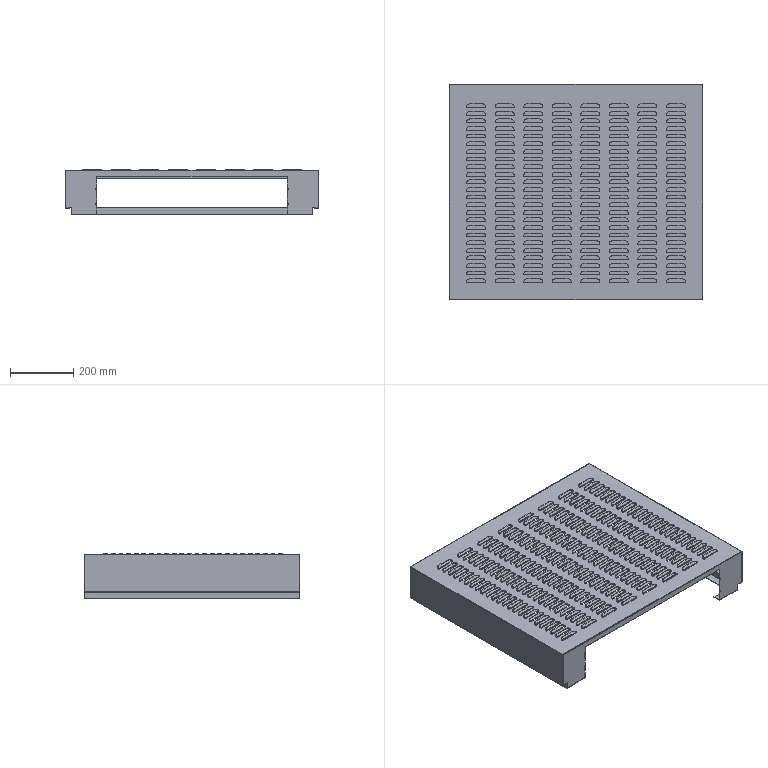Part | STEP file | HESS-408-70-15W-W-22-lower door frame | 1 solid | 2822 faces | box 800 x 681 x 144 mm | volume 1412616 mm3 | plane 2024 | cylinder 798 | commonest cylinder face diameters 17 x384 20 x384 0.2 x13 3.2 x13 10 x4